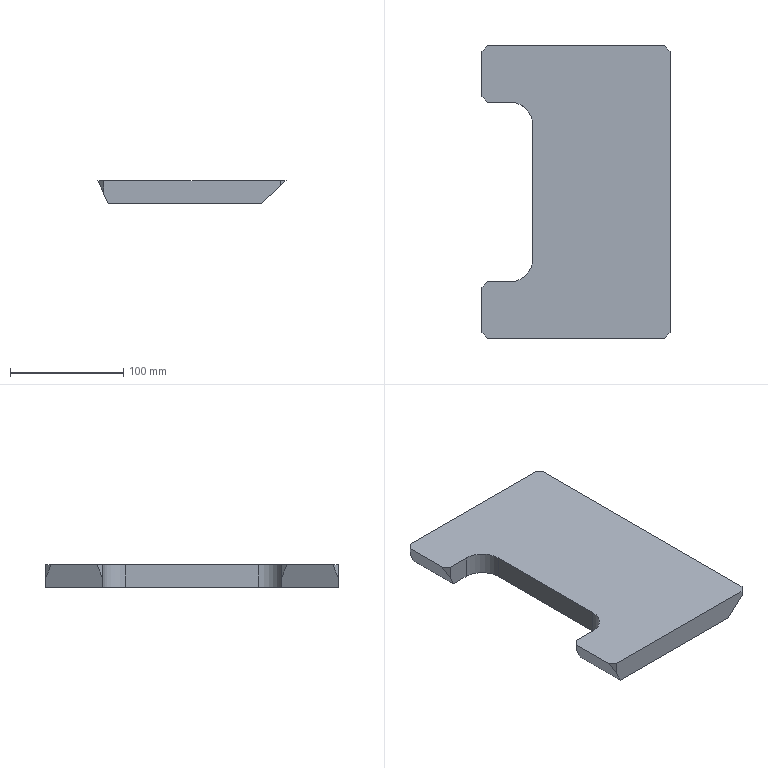Part | SolidWorks | features Extrusion 1, ICE 1 | 1 solid | 18 faces | box 166 x 258 x 20 mm | volume 651811 mm3 | plane 16 | cylinder 2 | commonest cylinder face diameters 40 x2
STEP:
#1=CARTESIAN_POINT('',(161.,0.,20.));
#2=VERTEX_POINT('',#1);
#3=CARTESIAN_POINT('',(161.,0.,15.455));
#4=VERTEX_POINT('',#3);
#5=CARTESIAN_POINT('',(161.,0.,20.));
#6=DIRECTION('',(0.,0.,-1.));
#7=VECTOR('',#6,1000.);
#8=LINE('',#5,#7);
#9=EDGE_CURVE('',#2,#4,#8,.T.);
#10=ORIENTED_EDGE('',*,*,#9,.T.);
#11=CARTESIAN_POINT('',(166.,5.,20.));
#12=VERTEX_POINT('',#11);
#13=CARTESIAN_POINT('',(162.462,1.462,16.784));
#14=DIRECTION('',(0.5948,0.5948,0.5407));
#15=VECTOR('',#14,1000.);
#16=LINE('',#13,#15);
#17=EDGE_CURVE('',#4,#12,#16,.T.);
#18=ORIENTED_EDGE('',*,*,#17,.T.);
#19=CARTESIAN_POINT('',(161.,0.,20.));
#20=DIRECTION('',(0.7071,0.7071,0.));
#21=VECTOR('',#20,1000.);
#22=LINE('',#19,#21);
#23=EDGE_CURVE('',#2,#12,#22,.T.);
#24=ORIENTED_EDGE('',*,*,#23,.F.);
#25=EDGE_LOOP('',(#10,#18,#24));
#26=FACE_OUTER_BOUND('',#25,.T.);
#27=CARTESIAN_POINT('',(161.,0.,20.));
#28=DIRECTION('',(-0.7071,0.7071,0.));
#29=DIRECTION('',(-0.7071,-0.7071,0.));
#30=AXIS2_PLACEMENT_3D('',#27,#28,#29);
#31=PLANE('',#30);
#32=ADVANCED_FACE('',(#26),#31,.F.);
#33=CARTESIAN_POINT('',(166.,253.,20.));
#34=VERTEX_POINT('',#33);
#35=CARTESIAN_POINT('',(161.,258.,20.));
#36=VERTEX_POINT('',#35);
#37=CARTESIAN_POINT('',(166.,253.,20.));
#38=DIRECTION('',(-0.7071,0.7071,0.));
#39=VECTOR('',#38,1000.);
#40=LINE('',#37,#39);
#41=EDGE_CURVE('',#34,#36,#40,.T.);
#42=ORIENTED_EDGE('',*,*,#41,.F.);
#43=CARTESIAN_POINT('',(161.,258.,15.455));
#44=VERTEX_POINT('',#43);
#45=CARTESIAN_POINT('',(166.,253.,20.));
#46=DIRECTION('',(-0.5948,0.5948,-0.5407));
#47=VECTOR('',#46,1000.);
#48=LINE('',#45,#47);
#49=EDGE_CURVE('',#34,#44,#48,.T.);
#50=ORIENTED_EDGE('',*,*,#49,.T.);
#51=CARTESIAN_POINT('',(161.,258.,20.));
#52=DIRECTION('',(0.,0.,-1.));
#53=VECTOR('',#52,1000.);
#54=LINE('',#51,#53);
#55=EDGE_CURVE('',#36,#44,#54,.T.);
#56=ORIENTED_EDGE('',*,*,#55,.F.);
#57=EDGE_LOOP('',(#42,#50,#56));
#58=FACE_OUTER_BOUND('',#57,.T.);
#59=CARTESIAN_POINT('',(166.,253.,20.));
#60=DIRECTION('',(-0.7071,-0.7071,0.));
#61=DIRECTION('',(0.7071,-0.7071,0.));
#62=AXIS2_PLACEMENT_3D('',#59,#60,#61);
#63=PLANE('',#62);
#64=ADVANCED_FACE('',(#58),#63,.F.);
#65=ORIENTED_EDGE('',*,*,#55,.T.);
#66=CARTESIAN_POINT('',(144.,258.,0.));
#67=VERTEX_POINT('',#66);
#68=CARTESIAN_POINT('',(166.,258.,20.));
#69=DIRECTION('',(-0.7399,0.,-0.6727));
#70=VECTOR('',#69,1000.);
#71=LINE('',#68,#70);
#72=EDGE_CURVE('',#44,#67,#71,.T.);
#73=ORIENTED_EDGE('',*,*,#72,.T.);
#74=CARTESIAN_POINT('',(9.,258.,0.));
#75=VERTEX_POINT('',#74);
#76=CARTESIAN_POINT('',(5.,258.,0.));
#77=DIRECTION('',(-1.,0.,0.));
#78=VECTOR('',#77,1000.);
#79=LINE('',#76,#78);
#80=EDGE_CURVE('',#67,#75,#79,.T.);
#81=ORIENTED_EDGE('',*,*,#80,.T.);
#82=CARTESIAN_POINT('',(5.,258.,8.889));
#83=VERTEX_POINT('',#82);
#84=CARTESIAN_POINT('',(0.,258.,20.));
#85=DIRECTION('',(-0.4104,0.,0.9119));
#86=VECTOR('',#85,1000.);
#87=LINE('',#84,#86);
#88=EDGE_CURVE('',#75,#83,#87,.T.);
#89=ORIENTED_EDGE('',*,*,#88,.T.);
#90=CARTESIAN_POINT('',(5.,258.,20.));
#91=VERTEX_POINT('',#90);
#92=CARTESIAN_POINT('',(5.,258.,20.));
#93=DIRECTION('',(0.,0.,-1.));
#94=VECTOR('',#93,1000.);
#95=LINE('',#92,#94);
#96=EDGE_CURVE('',#91,#83,#95,.T.);
#97=ORIENTED_EDGE('',*,*,#96,.F.);
#98=CARTESIAN_POINT('',(5.,258.,20.));
#99=DIRECTION('',(-1.,0.,0.));
#100=VECTOR('',#99,1000.);
#101=LINE('',#98,#100);
#102=EDGE_CURVE('',#36,#91,#101,.T.);
#103=ORIENTED_EDGE('',*,*,#102,.F.);
#104=EDGE_LOOP('',(#65,#73,#81,#89,#97,#103));
#105=FACE_OUTER_BOUND('',#104,.T.);
#106=CARTESIAN_POINT('',(5.,258.,20.));
#107=DIRECTION('',(0.,-1.,0.));
#108=DIRECTION('',(0.,0.,-1.));
#109=AXIS2_PLACEMENT_3D('',#106,#107,#108);
#110=PLANE('',#109);
#111=ADVANCED_FACE('',(#105),#110,.F.);
#112=ORIENTED_EDGE('',*,*,#96,.T.);
#113=CARTESIAN_POINT('',(0.,253.,20.));
#114=VERTEX_POINT('',#113);
#115=CARTESIAN_POINT('',(0.,253.,20.));
#116=DIRECTION('',(-0.3796,-0.3796,0.8436));
#117=VECTOR('',#116,1000.);
#118=LINE('',#115,#117);
#119=EDGE_CURVE('',#83,#114,#118,.T.);
#120=ORIENTED_EDGE('',*,*,#119,.T.);
#121=CARTESIAN_POINT('',(0.,253.,20.));
#122=DIRECTION('',(-0.7071,-0.7071,0.));
#123=VECTOR('',#122,1000.);
#124=LINE('',#121,#123);
#125=EDGE_CURVE('',#91,#114,#124,.T.);
#126=ORIENTED_EDGE('',*,*,#125,.F.);
#127=EDGE_LOOP('',(#112,#120,#126));
#128=FACE_OUTER_BOUND('',#127,.T.);
#129=CARTESIAN_POINT('',(0.,253.,20.));
#130=DIRECTION('',(0.7071,-0.7071,0.));
#131=DIRECTION('',(0.7071,0.7071,0.));
#132=AXIS2_PLACEMENT_3D('',#129,#130,#131);
#133=PLANE('',#132);
#134=ADVANCED_FACE('',(#128),#133,.F.);
#135=CARTESIAN_POINT('',(0.,213.,20.));
#136=VERTEX_POINT('',#135);
#137=CARTESIAN_POINT('',(5.,208.,20.));
#138=VERTEX_POINT('',#137);
#139=CARTESIAN_POINT('',(0.,213.,20.));
#140=DIRECTION('',(0.7071,-0.7071,0.));
#141=VECTOR('',#140,1000.);
#142=LINE('',#139,#141);
#143=EDGE_CURVE('',#136,#138,#142,.T.);
#144=ORIENTED_EDGE('',*,*,#143,.F.);
#145=CARTESIAN_POINT('',(5.,208.,8.889));
#146=VERTEX_POINT('',#145);
#147=CARTESIAN_POINT('',(0.,213.,20.));
#148=DIRECTION('',(0.3796,-0.3796,-0.8436));
#149=VECTOR('',#148,1000.);
#150=LINE('',#147,#149);
#151=EDGE_CURVE('',#136,#146,#150,.T.);
#152=ORIENTED_EDGE('',*,*,#151,.T.);
#153=CARTESIAN_POINT('',(5.,208.,20.));
#154=DIRECTION('',(0.,0.,-1.));
#155=VECTOR('',#154,1000.);
#156=LINE('',#153,#155);
#157=EDGE_CURVE('',#138,#146,#156,.T.);
#158=ORIENTED_EDGE('',*,*,#157,.F.);
#159=EDGE_LOOP('',(#144,#152,#158));
#160=FACE_OUTER_BOUND('',#159,.T.);
#161=CARTESIAN_POINT('',(0.,213.,20.));
#162=DIRECTION('',(0.7071,0.7071,0.));
#163=DIRECTION('',(-0.7071,0.7071,0.));
#164=AXIS2_PLACEMENT_3D('',#161,#162,#163);
#165=PLANE('',#164);
#166=ADVANCED_FACE('',(#160),#165,.F.);
#167=ORIENTED_EDGE('',*,*,#157,.T.);
#168=CARTESIAN_POINT('',(9.,208.,0.));
#169=VERTEX_POINT('',#168);
#170=CARTESIAN_POINT('',(0.842,208.,18.129));
#171=DIRECTION('',(0.4104,0.,-0.9119));
#172=VECTOR('',#171,1000.);
#173=LINE('',#170,#172);
#174=EDGE_CURVE('',#146,#169,#173,.T.);
#175=ORIENTED_EDGE('',*,*,#174,.T.);
#176=CARTESIAN_POINT('',(25.,208.,0.));
#177=VERTEX_POINT('',#176);
#178=CARTESIAN_POINT('',(5.,208.,0.));
#179=DIRECTION('',(1.,0.,0.));
#180=VECTOR('',#179,1000.);
#181=LINE('',#178,#180);
#182=EDGE_CURVE('',#169,#177,#181,.T.);
#183=ORIENTED_EDGE('',*,*,#182,.T.);
#184=CARTESIAN_POINT('',(25.,208.,20.));
#185=VERTEX_POINT('',#184);
#186=CARTESIAN_POINT('',(25.,208.,20.));
#187=DIRECTION('',(0.,0.,-1.));
#188=VECTOR('',#187,1000.);
#189=LINE('',#186,#188);
#190=EDGE_CURVE('',#185,#177,#189,.T.);
#191=ORIENTED_EDGE('',*,*,#190,.F.);
#192=CARTESIAN_POINT('',(5.,208.,20.));
#193=DIRECTION('',(1.,0.,0.));
#194=VECTOR('',#193,1000.);
#195=LINE('',#192,#194);
#196=EDGE_CURVE('',#138,#185,#195,.T.);
#197=ORIENTED_EDGE('',*,*,#196,.F.);
#198=EDGE_LOOP('',(#167,#175,#183,#191,#197));
#199=FACE_OUTER_BOUND('',#198,.T.);
#200=CARTESIAN_POINT('',(5.,208.,20.));
#201=DIRECTION('',(0.,1.,0.));
#202=DIRECTION('',(0.,0.,1.));
#203=AXIS2_PLACEMENT_3D('',#200,#201,#202);
#204=PLANE('',#203);
#205=ADVANCED_FACE('',(#199),#204,.F.);
#206=CARTESIAN_POINT('',(45.,188.,0.));
#207=VERTEX_POINT('',#206);
#208=CARTESIAN_POINT('',(25.,188.,0.));
#209=DIRECTION('',(0.,0.,-1.));
#210=DIRECTION('',(-1.,0.,0.));
#211=AXIS2_PLACEMENT_3D('',#208,#209,#210);
#212=CIRCLE('',#211,20.);
#213=EDGE_CURVE('',#177,#207,#212,.T.);
#214=ORIENTED_EDGE('',*,*,#213,.T.);
#215=CARTESIAN_POINT('',(45.,188.,20.));
#216=VERTEX_POINT('',#215);
#217=CARTESIAN_POINT('',(45.,188.,20.));
#218=DIRECTION('',(0.,0.,-1.));
#219=VECTOR('',#218,1000.);
#220=LINE('',#217,#219);
#221=EDGE_CURVE('',#216,#207,#220,.T.);
#222=ORIENTED_EDGE('',*,*,#221,.F.);
#223=CARTESIAN_POINT('',(25.,188.,20.));
#224=DIRECTION('',(0.,0.,-1.));
#225=DIRECTION('',(-1.,0.,0.));
#226=AXIS2_PLACEMENT_3D('',#223,#224,#225);
#227=CIRCLE('',#226,20.);
#228=EDGE_CURVE('',#185,#216,#227,.T.);
#229=ORIENTED_EDGE('',*,*,#228,.F.);
#230=ORIENTED_EDGE('',*,*,#190,.T.);
#231=EDGE_LOOP('',(#214,#222,#229,#230));
#232=FACE_OUTER_BOUND('',#231,.T.);
#233=CARTESIAN_POINT('',(25.,188.,20.));
#234=DIRECTION('',(0.,0.,-1.));
#235=DIRECTION('',(-1.,0.,0.));
#236=AXIS2_PLACEMENT_3D('',#233,#234,#235);
#237=CYLINDRICAL_SURFACE('',#236,20.);
#238=ADVANCED_FACE('',(#232),#237,.F.);
#239=CARTESIAN_POINT('',(45.,70.,0.));
#240=VERTEX_POINT('',#239);
#241=CARTESIAN_POINT('',(45.,188.,0.));
#242=DIRECTION('',(0.,-1.,0.));
#243=VECTOR('',#242,1000.);
#244=LINE('',#241,#243);
#245=EDGE_CURVE('',#207,#240,#244,.T.);
#246=ORIENTED_EDGE('',*,*,#245,.T.);
#247=CARTESIAN_POINT('',(45.,70.,20.));
#248=VERTEX_POINT('',#247);
#249=CARTESIAN_POINT('',(45.,70.,20.));
#250=DIRECTION('',(0.,0.,-1.));
#251=VECTOR('',#250,1000.);
#252=LINE('',#249,#251);
#253=EDGE_CURVE('',#248,#240,#252,.T.);
#254=ORIENTED_EDGE('',*,*,#253,.F.);
#255=CARTESIAN_POINT('',(45.,188.,20.));
#256=DIRECTION('',(0.,-1.,0.));
#257=VECTOR('',#256,1000.);
#258=LINE('',#255,#257);
#259=EDGE_CURVE('',#216,#248,#258,.T.);
#260=ORIENTED_EDGE('',*,*,#259,.F.);
#261=ORIENTED_EDGE('',*,*,#221,.T.);
#262=EDGE_LOOP('',(#246,#254,#260,#261));
#263=FACE_OUTER_BOUND('',#262,.T.);
#264=CARTESIAN_POINT('',(45.,188.,20.));
#265=DIRECTION('',(1.,0.,0.));
#266=DIRECTION('',(0.,1.,0.));
#267=AXIS2_PLACEMENT_3D('',#264,#265,#266);
#268=PLANE('',#267);
#269=ADVANCED_FACE('',(#263),#268,.F.);
#270=CARTESIAN_POINT('',(25.,50.,0.));
#271=VERTEX_POINT('',#270);
#272=CARTESIAN_POINT('',(25.,70.,0.));
#273=DIRECTION('',(0.,0.,-1.));
#274=DIRECTION('',(1.,0.,0.));
#275=AXIS2_PLACEMENT_3D('',#272,#273,#274);
#276=CIRCLE('',#275,20.);
#277=EDGE_CURVE('',#240,#271,#276,.T.);
#278=ORIENTED_EDGE('',*,*,#277,.T.);
#279=CARTESIAN_POINT('',(25.,50.,20.));
#280=VERTEX_POINT('',#279);
#281=CARTESIAN_POINT('',(25.,50.,20.));
#282=DIRECTION('',(0.,0.,-1.));
#283=VECTOR('',#282,1000.);
#284=LINE('',#281,#283);
#285=EDGE_CURVE('',#280,#271,#284,.T.);
#286=ORIENTED_EDGE('',*,*,#285,.F.);
#287=CARTESIAN_POINT('',(25.,70.,20.));
#288=DIRECTION('',(0.,0.,-1.));
#289=DIRECTION('',(1.,0.,0.));
#290=AXIS2_PLACEMENT_3D('',#287,#288,#289);
#291=CIRCLE('',#290,20.);
#292=EDGE_CURVE('',#248,#280,#291,.T.);
#293=ORIENTED_EDGE('',*,*,#292,.F.);
#294=ORIENTED_EDGE('',*,*,#253,.T.);
#295=EDGE_LOOP('',(#278,#286,#293,#294));
#296=FACE_OUTER_BOUND('',#295,.T.);
#297=CARTESIAN_POINT('',(25.,70.,20.));
#298=DIRECTION('',(0.,0.,-1.));
#299=DIRECTION('',(-1.,0.,0.));
#300=AXIS2_PLACEMENT_3D('',#297,#298,#299);
#301=CYLINDRICAL_SURFACE('',#300,20.);
#302=ADVANCED_FACE('',(#296),#301,.F.);
#303=CARTESIAN_POINT('',(9.,50.,0.));
#304=VERTEX_POINT('',#303);
#305=CARTESIAN_POINT('',(5.,50.,0.));
#306=DIRECTION('',(-1.,0.,0.));
#307=VECTOR('',#306,1000.);
#308=LINE('',#305,#307);
#309=EDGE_CURVE('',#271,#304,#308,.T.);
#310=ORIENTED_EDGE('',*,*,#309,.T.);
#311=CARTESIAN_POINT('',(5.,50.,8.889));
#312=VERTEX_POINT('',#311);
#313=CARTESIAN_POINT('',(0.842,50.,18.129));
#314=DIRECTION('',(-0.4104,0.,0.9119));
#315=VECTOR('',#314,1000.);
#316=LINE('',#313,#315);
#317=EDGE_CURVE('',#304,#312,#316,.T.);
#318=ORIENTED_EDGE('',*,*,#317,.T.);
#319=CARTESIAN_POINT('',(5.,50.,20.));
#320=VERTEX_POINT('',#319);
#321=CARTESIAN_POINT('',(5.,50.,20.));
#322=DIRECTION('',(0.,0.,-1.));
#323=VECTOR('',#322,1000.);
#324=LINE('',#321,#323);
#325=EDGE_CURVE('',#320,#312,#324,.T.);
#326=ORIENTED_EDGE('',*,*,#325,.F.);
#327=CARTESIAN_POINT('',(5.,50.,20.));
#328=DIRECTION('',(-1.,0.,0.));
#329=VECTOR('',#328,1000.);
#330=LINE('',#327,#329);
#331=EDGE_CURVE('',#280,#320,#330,.T.);
#332=ORIENTED_EDGE('',*,*,#331,.F.);
#333=ORIENTED_EDGE('',*,*,#285,.T.);
#334=EDGE_LOOP('',(#310,#318,#326,#332,#333));
#335=FACE_OUTER_BOUND('',#334,.T.);
#336=CARTESIAN_POINT('',(5.,50.,20.));
#337=DIRECTION('',(0.,-1.,0.));
#338=DIRECTION('',(1.,0.,0.));
#339=AXIS2_PLACEMENT_3D('',#336,#337,#338);
#340=PLANE('',#339);
#341=ADVANCED_FACE('',(#335),#340,.F.);
#342=ORIENTED_EDGE('',*,*,#325,.T.);
#343=CARTESIAN_POINT('',(0.,45.,20.));
#344=VERTEX_POINT('',#343);
#345=CARTESIAN_POINT('',(0.,45.,20.));
#346=DIRECTION('',(-0.3796,-0.3796,0.8436));
#347=VECTOR('',#346,1000.);
#348=LINE('',#345,#347);
#349=EDGE_CURVE('',#312,#344,#348,.T.);
#350=ORIENTED_EDGE('',*,*,#349,.T.);
#351=CARTESIAN_POINT('',(0.,45.,20.));
#352=DIRECTION('',(-0.7071,-0.7071,0.));
#353=VECTOR('',#352,1000.);
#354=LINE('',#351,#353);
#355=EDGE_CURVE('',#320,#344,#354,.T.);
#356=ORIENTED_EDGE('',*,*,#355,.F.);
#357=EDGE_LOOP('',(#342,#350,#356));
#358=FACE_OUTER_BOUND('',#357,.T.);
#359=CARTESIAN_POINT('',(0.,45.,20.));
#360=DIRECTION('',(0.7071,-0.7071,0.));
#361=DIRECTION('',(0.7071,0.7071,0.));
#362=AXIS2_PLACEMENT_3D('',#359,#360,#361);
#363=PLANE('',#362);
#364=ADVANCED_FACE('',(#358),#363,.F.);
#365=CARTESIAN_POINT('',(0.,5.,20.));
#366=VERTEX_POINT('',#365);
#367=CARTESIAN_POINT('',(5.,0.,20.));
#368=VERTEX_POINT('',#367);
#369=CARTESIAN_POINT('',(0.,5.,20.));
#370=DIRECTION('',(0.7071,-0.7071,0.));
#371=VECTOR('',#370,1000.);
#372=LINE('',#369,#371);
#373=EDGE_CURVE('',#366,#368,#372,.T.);
#374=ORIENTED_EDGE('',*,*,#373,.F.);
#375=CARTESIAN_POINT('',(5.,0.,8.889));
#376=VERTEX_POINT('',#375);
#377=CARTESIAN_POINT('',(0.,5.,20.));
#378=DIRECTION('',(0.3796,-0.3796,-0.8436));
#379=VECTOR('',#378,1000.);
#380=LINE('',#377,#379);
#381=EDGE_CURVE('',#366,#376,#380,.T.);
#382=ORIENTED_EDGE('',*,*,#381,.T.);
#383=CARTESIAN_POINT('',(5.,0.,20.));
#384=DIRECTION('',(0.,0.,-1.));
#385=VECTOR('',#384,1000.);
#386=LINE('',#383,#385);
#387=EDGE_CURVE('',#368,#376,#386,.T.);
#388=ORIENTED_EDGE('',*,*,#387,.F.);
#389=EDGE_LOOP('',(#374,#382,#388));
#390=FACE_OUTER_BOUND('',#389,.T.);
#391=CARTESIAN_POINT('',(0.,5.,20.));
#392=DIRECTION('',(0.7071,0.7071,0.));
#393=DIRECTION('',(-0.7071,0.7071,0.));
#394=AXIS2_PLACEMENT_3D('',#391,#392,#393);
#395=PLANE('',#394);
#396=ADVANCED_FACE('',(#390),#395,.F.);
#397=CARTESIAN_POINT('',(9.,0.,0.));
#398=VERTEX_POINT('',#397);
#399=CARTESIAN_POINT('',(144.,0.,0.));
#400=VERTEX_POINT('',#399);
#401=CARTESIAN_POINT('',(5.,0.,0.));
#402=DIRECTION('',(1.,0.,0.));
#403=VECTOR('',#402,1000.);
#404=LINE('',#401,#403);
#405=EDGE_CURVE('',#398,#400,#404,.T.);
#406=ORIENTED_EDGE('',*,*,#405,.T.);
#407=CARTESIAN_POINT('',(166.,0.,20.));
#408=DIRECTION('',(-0.7399,0.,-0.6727));
#409=VECTOR('',#408,1000.);
#410=LINE('',#407,#409);
#411=EDGE_CURVE('',#4,#400,#410,.T.);
#412=ORIENTED_EDGE('',*,*,#411,.F.);
#413=ORIENTED_EDGE('',*,*,#9,.F.);
#414=CARTESIAN_POINT('',(5.,0.,20.));
#415=DIRECTION('',(1.,0.,0.));
#416=VECTOR('',#415,1000.);
#417=LINE('',#414,#416);
#418=EDGE_CURVE('',#368,#2,#417,.T.);
#419=ORIENTED_EDGE('',*,*,#418,.F.);
#420=ORIENTED_EDGE('',*,*,#387,.T.);
#421=CARTESIAN_POINT('',(0.,0.,20.));
#422=DIRECTION('',(-0.4104,0.,0.9119));
#423=VECTOR('',#422,1000.);
#424=LINE('',#421,#423);
#425=EDGE_CURVE('',#398,#376,#424,.T.);
#426=ORIENTED_EDGE('',*,*,#425,.F.);
#427=EDGE_LOOP('',(#406,#412,#413,#419,#420,#426));
#428=FACE_OUTER_BOUND('',#427,.T.);
#429=CARTESIAN_POINT('',(5.,0.,20.));
#430=DIRECTION('',(0.,1.,0.));
#431=DIRECTION('',(0.,0.,1.));
#432=AXIS2_PLACEMENT_3D('',#429,#430,#431);
#433=PLANE('',#432);
#434=ADVANCED_FACE('',(#428),#433,.F.);
#435=ORIENTED_EDGE('',*,*,#23,.T.);
#436=CARTESIAN_POINT('',(166.,5.,20.));
#437=DIRECTION('',(0.,1.,0.));
#438=VECTOR('',#437,1000.);
#439=LINE('',#436,#438);
#440=EDGE_CURVE('',#12,#34,#439,.T.);
#441=ORIENTED_EDGE('',*,*,#440,.T.);
#442=ORIENTED_EDGE('',*,*,#41,.T.);
#443=ORIENTED_EDGE('',*,*,#102,.T.);
#444=ORIENTED_EDGE('',*,*,#125,.T.);
#445=CARTESIAN_POINT('',(0.,253.,20.));
#446=DIRECTION('',(0.,-1.,0.));
#447=VECTOR('',#446,1000.);
#448=LINE('',#445,#447);
#449=EDGE_CURVE('',#114,#136,#448,.T.);
#450=ORIENTED_EDGE('',*,*,#449,.T.);
#451=ORIENTED_EDGE('',*,*,#143,.T.);
#452=ORIENTED_EDGE('',*,*,#196,.T.);
#453=ORIENTED_EDGE('',*,*,#228,.T.);
#454=ORIENTED_EDGE('',*,*,#259,.T.);
#455=ORIENTED_EDGE('',*,*,#292,.T.);
#456=ORIENTED_EDGE('',*,*,#331,.T.);
#457=ORIENTED_EDGE('',*,*,#355,.T.);
#458=CARTESIAN_POINT('',(0.,5.,20.));
#459=DIRECTION('',(0.,-1.,0.));
#460=VECTOR('',#459,1000.);
#461=LINE('',#458,#460);
#462=EDGE_CURVE('',#344,#366,#461,.T.);
#463=ORIENTED_EDGE('',*,*,#462,.T.);
#464=ORIENTED_EDGE('',*,*,#373,.T.);
#465=ORIENTED_EDGE('',*,*,#418,.T.);
#466=EDGE_LOOP('',(#435,#441,#442,#443,#444,#450,#451,#452,#453,#454,#455,#456,#457,#463,#464,#465));
#467=FACE_OUTER_BOUND('',#466,.T.);
#468=CARTESIAN_POINT('',(25.,188.,20.));
#469=DIRECTION('',(0.,0.,-1.));
#470=DIRECTION('',(-1.,0.,0.));
#471=AXIS2_PLACEMENT_3D('',#468,#469,#470);
#472=PLANE('',#471);
#473=ADVANCED_FACE('',(#467),#472,.F.);
#474=CARTESIAN_POINT('',(144.,258.,0.));
#475=DIRECTION('',(0.,-1.,0.));
#476=VECTOR('',#475,1000.);
#477=LINE('',#474,#476);
#478=EDGE_CURVE('',#67,#400,#477,.T.);
#479=ORIENTED_EDGE('',*,*,#478,.T.);
#480=ORIENTED_EDGE('',*,*,#405,.F.);
#481=CARTESIAN_POINT('',(9.,188.,0.));
#482=DIRECTION('',(0.,-1.,0.));
#483=VECTOR('',#482,1000.);
#484=LINE('',#481,#483);
#485=EDGE_CURVE('',#304,#398,#484,.T.);
#486=ORIENTED_EDGE('',*,*,#485,.F.);
#487=ORIENTED_EDGE('',*,*,#309,.F.);
#488=ORIENTED_EDGE('',*,*,#277,.F.);
#489=ORIENTED_EDGE('',*,*,#245,.F.);
#490=ORIENTED_EDGE('',*,*,#213,.F.);
#491=ORIENTED_EDGE('',*,*,#182,.F.);
#492=CARTESIAN_POINT('',(9.,258.,0.));
#493=DIRECTION('',(0.,-1.,0.));
#494=VECTOR('',#493,1000.);
#495=LINE('',#492,#494);
#496=EDGE_CURVE('',#75,#169,#495,.T.);
#497=ORIENTED_EDGE('',*,*,#496,.F.);
#498=ORIENTED_EDGE('',*,*,#80,.F.);
#499=EDGE_LOOP('',(#479,#480,#486,#487,#488,#489,#490,#491,#497,#498));
#500=FACE_OUTER_BOUND('',#499,.T.);
#501=CARTESIAN_POINT('',(25.,188.,0.));
#502=DIRECTION('',(0.,0.,-1.));
#503=DIRECTION('',(-1.,0.,0.));
#504=AXIS2_PLACEMENT_3D('',#501,#502,#503);
#505=PLANE('',#504);
#506=ADVANCED_FACE('',(#500),#505,.T.);
#507=ORIENTED_EDGE('',*,*,#485,.T.);
#508=ORIENTED_EDGE('',*,*,#425,.T.);
#509=ORIENTED_EDGE('',*,*,#381,.F.);
#510=ORIENTED_EDGE('',*,*,#462,.F.);
#511=ORIENTED_EDGE('',*,*,#349,.F.);
#512=ORIENTED_EDGE('',*,*,#317,.F.);
#513=EDGE_LOOP('',(#507,#508,#509,#510,#511,#512));
#514=FACE_OUTER_BOUND('',#513,.T.);
#515=CARTESIAN_POINT('',(0.,258.,20.));
#516=DIRECTION('',(0.9119,0.,0.4104));
#517=DIRECTION('',(0.4104,0.,-0.9119));
#518=AXIS2_PLACEMENT_3D('',#515,#516,#517);
#519=PLANE('',#518);
#520=ADVANCED_FACE('',(#514),#519,.F.);
#521=ORIENTED_EDGE('',*,*,#88,.F.);
#522=ORIENTED_EDGE('',*,*,#496,.T.);
#523=ORIENTED_EDGE('',*,*,#174,.F.);
#524=ORIENTED_EDGE('',*,*,#151,.F.);
#525=ORIENTED_EDGE('',*,*,#449,.F.);
#526=ORIENTED_EDGE('',*,*,#119,.F.);
#527=EDGE_LOOP('',(#521,#522,#523,#524,#525,#526));
#528=FACE_OUTER_BOUND('',#527,.T.);
#529=CARTESIAN_POINT('',(0.,258.,20.));
#530=DIRECTION('',(0.9119,0.,0.4104));
#531=DIRECTION('',(0.4104,0.,-0.9119));
#532=AXIS2_PLACEMENT_3D('',#529,#530,#531);
#533=PLANE('',#532);
#534=ADVANCED_FACE('',(#528),#533,.F.);
#535=ORIENTED_EDGE('',*,*,#411,.T.);
#536=ORIENTED_EDGE('',*,*,#478,.F.);
#537=ORIENTED_EDGE('',*,*,#72,.F.);
#538=ORIENTED_EDGE('',*,*,#49,.F.);
#539=ORIENTED_EDGE('',*,*,#440,.F.);
#540=ORIENTED_EDGE('',*,*,#17,.F.);
#541=EDGE_LOOP('',(#535,#536,#537,#538,#539,#540));
#542=FACE_OUTER_BOUND('',#541,.T.);
#543=CARTESIAN_POINT('',(166.,258.,20.));
#544=DIRECTION('',(-0.6727,0.,0.7399));
#545=DIRECTION('',(0.7399,0.,0.6727));
#546=AXIS2_PLACEMENT_3D('',#543,#544,#545);
#547=PLANE('',#546);
#548=ADVANCED_FACE('',(#542),#547,.F.);
#549=CLOSED_SHELL('',(#32,#64,#111,#134,#166,#205,#238,#269,#302,#341,#364,#396,#434,#473,#506,#520,#534,#548));
#550=MANIFOLD_SOLID_BREP('',#549);
#551=CARTESIAN_POINT('',(0.,0.,0.));
#552=DIRECTION('',(0.,0.,1.));
#553=DIRECTION('',(1.,0.,0.));
#554=AXIS2_PLACEMENT_3D('',#551,#552,#553);
#555=(LENGTH_UNIT()NAMED_UNIT(*)SI_UNIT(.MILLI.,.METRE.));
#556=UNCERTAINTY_MEASURE_WITH_UNIT(LENGTH_MEASURE(0.00001),#555,'','');
#557=(NAMED_UNIT(*)PLANE_ANGLE_UNIT()SI_UNIT($,.RADIAN.));
#558=(NAMED_UNIT(*)SI_UNIT($,.STERADIAN.)SOLID_ANGLE_UNIT());
#559=(GEOMETRIC_REPRESENTATION_CONTEXT(3)GLOBAL_UNCERTAINTY_ASSIGNED_CONTEXT((#556))GLOBAL_UNIT_ASSIGNED_CONTEXT((#555,#557,#558))REPRESENTATION_CONTEXT('',''));
#560=ADVANCED_BREP_SHAPE_REPRESENTATION('',(#550,#554),#559);